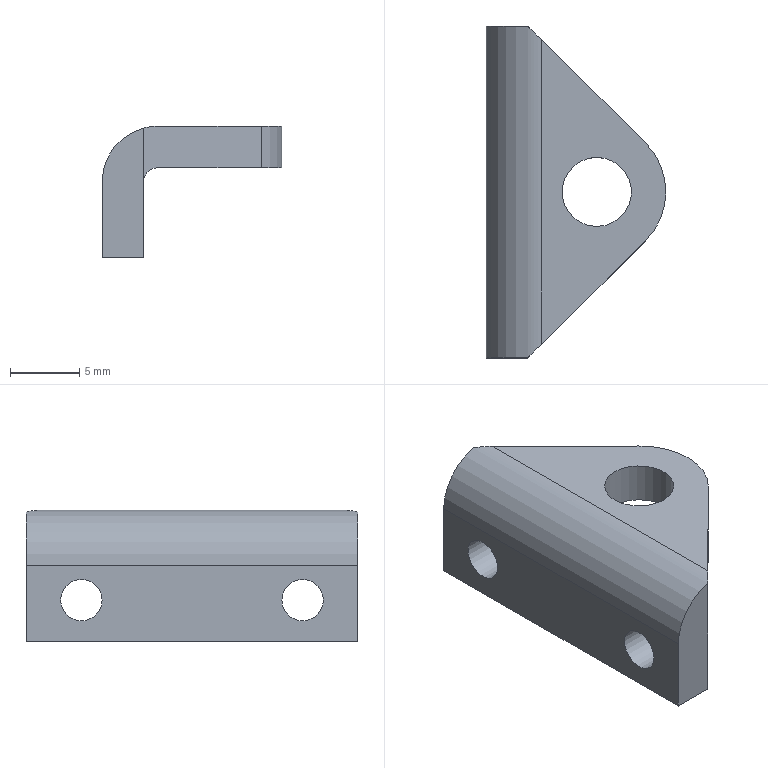Part | STEP file | 1-40.8 | 1 solid | 15 faces | box 13 x 24 x 9.5 mm | volume 924.566 mm3 | plane 9 | cylinder 6 | commonest cylinder face diameters 3 x2 2 x1 5 x1 8 x1 10 x1
STEP:
#1=CARTESIAN_POINT('',(0.,0.,0.));
#2=DIRECTION('',(0.,0.,1.));
#3=DIRECTION('',(1.,0.,0.));
#4=AXIS2_PLACEMENT_3D('',#1,#2,#3);
#5=CARTESIAN_POINT('',(0.,-12.,-4.75));
#6=VERTEX_POINT('',#5);
#7=CARTESIAN_POINT('',(0.,12.,-4.75));
#8=VERTEX_POINT('',#7);
#9=CARTESIAN_POINT('',(0.,-12.,-4.75));
#10=DIRECTION('',(0.,1.,0.));
#11=VECTOR('',#10,1.);
#12=LINE('',#9,#11);
#13=CARTESIAN_POINT('',(1.5,0.,-4.75));
#14=DIRECTION('',(0.,0.,-1.));
#15=DIRECTION('',(0.,1.,0.));
#16=AXIS2_PLACEMENT_3D('',#13,#14,#15);
#17=PLANE('',#16);
#18=CARTESIAN_POINT('',(-12.,-1.5));
#19=DIRECTION('',(1.,0.));
#20=VECTOR('',#19,1.);
#21=LINE('',#18,#20);
#22=(GEOMETRIC_REPRESENTATION_CONTEXT(2)PARAMETRIC_REPRESENTATION_CONTEXT()REPRESENTATION_CONTEXT('',''));
#23=DEFINITIONAL_REPRESENTATION('',(#21),#22);
#24=PCURVE('',#17,#23);
#25=CARTESIAN_POINT('',(0.,0.,7.25));
#26=DIRECTION('',(1.,0.,0.));
#27=DIRECTION('',(0.,1.,0.));
#28=AXIS2_PLACEMENT_3D('',#25,#26,#27);
#29=PLANE('',#28);
#30=CARTESIAN_POINT('',(-12.,-12.));
#31=DIRECTION('',(1.,0.));
#32=VECTOR('',#31,1.);
#33=LINE('',#30,#32);
#34=(GEOMETRIC_REPRESENTATION_CONTEXT(2)PARAMETRIC_REPRESENTATION_CONTEXT()REPRESENTATION_CONTEXT('',''));
#35=DEFINITIONAL_REPRESENTATION('',(#33),#34);
#36=PCURVE('',#29,#35);
#37=SURFACE_CURVE('',#12,(#24,#36),.PCURVE_S1.);
#38=EDGE_CURVE('',#6,#8,#37,.T.);
#39=ORIENTED_EDGE('',*,*,#38,.T.);
#40=CARTESIAN_POINT('',(3.,12.,-4.75));
#41=VERTEX_POINT('',#40);
#42=CARTESIAN_POINT('',(0.,12.,-4.75));
#43=DIRECTION('',(1.,0.,0.));
#44=VECTOR('',#43,1.);
#45=LINE('',#42,#44);
#46=CARTESIAN_POINT('',(12.,-1.5));
#47=DIRECTION('',(0.,1.));
#48=VECTOR('',#47,1.);
#49=LINE('',#46,#48);
#50=(GEOMETRIC_REPRESENTATION_CONTEXT(2)PARAMETRIC_REPRESENTATION_CONTEXT()REPRESENTATION_CONTEXT('',''));
#51=DEFINITIONAL_REPRESENTATION('',(#49),#50);
#52=PCURVE('',#17,#51);
#53=CARTESIAN_POINT('',(-0.375,12.,2.75));
#54=DIRECTION('',(0.,1.,0.));
#55=DIRECTION('',(0.,0.,1.));
#56=AXIS2_PLACEMENT_3D('',#53,#54,#55);
#57=PLANE('',#56);
#58=CARTESIAN_POINT('',(-7.5,0.375));
#59=DIRECTION('',(0.,1.));
#60=VECTOR('',#59,1.);
#61=LINE('',#58,#60);
#62=(GEOMETRIC_REPRESENTATION_CONTEXT(2)PARAMETRIC_REPRESENTATION_CONTEXT()REPRESENTATION_CONTEXT('',''));
#63=DEFINITIONAL_REPRESENTATION('',(#61),#62);
#64=PCURVE('',#57,#63);
#65=SURFACE_CURVE('',#45,(#52,#64),.PCURVE_S1.);
#66=EDGE_CURVE('',#8,#41,#65,.T.);
#67=ORIENTED_EDGE('',*,*,#66,.T.);
#68=CARTESIAN_POINT('',(3.,-12.,-4.75));
#69=VERTEX_POINT('',#68);
#70=CARTESIAN_POINT('',(3.,-12.,-4.75));
#71=DIRECTION('',(0.,1.,0.));
#72=VECTOR('',#71,1.);
#73=LINE('',#70,#72);
#74=CARTESIAN_POINT('',(-12.,1.5));
#75=DIRECTION('',(1.,0.));
#76=VECTOR('',#75,1.);
#77=LINE('',#74,#76);
#78=(GEOMETRIC_REPRESENTATION_CONTEXT(2)PARAMETRIC_REPRESENTATION_CONTEXT()REPRESENTATION_CONTEXT('',''));
#79=DEFINITIONAL_REPRESENTATION('',(#77),#78);
#80=PCURVE('',#17,#79);
#81=CARTESIAN_POINT('',(3.,0.,7.25));
#82=DIRECTION('',(1.,0.,0.));
#83=DIRECTION('',(0.,1.,0.));
#84=AXIS2_PLACEMENT_3D('',#81,#82,#83);
#85=PLANE('',#84);
#86=CARTESIAN_POINT('',(-12.,-12.));
#87=DIRECTION('',(1.,0.));
#88=VECTOR('',#87,1.);
#89=LINE('',#86,#88);
#90=(GEOMETRIC_REPRESENTATION_CONTEXT(2)PARAMETRIC_REPRESENTATION_CONTEXT()REPRESENTATION_CONTEXT('',''));
#91=DEFINITIONAL_REPRESENTATION('',(#89),#90);
#92=PCURVE('',#85,#91);
#93=SURFACE_CURVE('',#73,(#80,#92),.PCURVE_S1.);
#94=EDGE_CURVE('',#69,#41,#93,.T.);
#95=ORIENTED_EDGE('',*,*,#94,.F.);
#96=CARTESIAN_POINT('',(0.,-12.,-4.75));
#97=DIRECTION('',(1.,0.,0.));
#98=VECTOR('',#97,1.);
#99=LINE('',#96,#98);
#100=CARTESIAN_POINT('',(-12.,-1.5));
#101=DIRECTION('',(0.,1.));
#102=VECTOR('',#101,1.);
#103=LINE('',#100,#102);
#104=(GEOMETRIC_REPRESENTATION_CONTEXT(2)PARAMETRIC_REPRESENTATION_CONTEXT()REPRESENTATION_CONTEXT('',''));
#105=DEFINITIONAL_REPRESENTATION('',(#103),#104);
#106=PCURVE('',#17,#105);
#107=CARTESIAN_POINT('',(-0.375,-12.,2.75));
#108=DIRECTION('',(0.,-1.,0.));
#109=DIRECTION('',(0.,0.,-1.));
#110=AXIS2_PLACEMENT_3D('',#107,#108,#109);
#111=PLANE('',#110);
#112=CARTESIAN_POINT('',(7.5,0.375));
#113=DIRECTION('',(0.,1.));
#114=VECTOR('',#113,1.);
#115=LINE('',#112,#114);
#116=(GEOMETRIC_REPRESENTATION_CONTEXT(2)PARAMETRIC_REPRESENTATION_CONTEXT()REPRESENTATION_CONTEXT('',''));
#117=DEFINITIONAL_REPRESENTATION('',(#115),#116);
#118=PCURVE('',#111,#117);
#119=SURFACE_CURVE('',#99,(#106,#118),.PCURVE_S1.);
#120=EDGE_CURVE('',#6,#69,#119,.T.);
#121=ORIENTED_EDGE('',*,*,#120,.F.);
#122=EDGE_LOOP('',(#39,#67,#95,#121));
#123=FACE_BOUND('',#122,.T.);
#124=ADVANCED_FACE('',(#123),#17,.T.);
#125=CARTESIAN_POINT('',(0.,-6.5,-1.75));
#126=VERTEX_POINT('',#125);
#127=CARTESIAN_POINT('',(3.,-6.5,-1.75));
#128=VERTEX_POINT('',#127);
#129=CARTESIAN_POINT('',(0.,-6.5,-1.75));
#130=DIRECTION('',(1.,0.,0.));
#131=VECTOR('',#130,1.);
#132=LINE('',#129,#131);
#133=CARTESIAN_POINT('',(0.,-8.,-1.75));
#134=DIRECTION('',(1.,0.,0.));
#135=DIRECTION('',(0.,1.,0.));
#136=AXIS2_PLACEMENT_3D('',#133,#134,#135);
#137=CYLINDRICAL_SURFACE('',#136,1.5);
#138=CARTESIAN_POINT('',(6.283,0.));
#139=DIRECTION('',(0.,1.));
#140=VECTOR('',#139,1.);
#141=LINE('',#138,#140);
#142=(GEOMETRIC_REPRESENTATION_CONTEXT(2)PARAMETRIC_REPRESENTATION_CONTEXT()REPRESENTATION_CONTEXT('',''));
#143=DEFINITIONAL_REPRESENTATION('',(#141),#142);
#144=PCURVE('',#137,#143);
#145=CARTESIAN_POINT('',(0.,0.));
#146=DIRECTION('',(0.,1.));
#147=VECTOR('',#146,1.);
#148=LINE('',#145,#147);
#149=(GEOMETRIC_REPRESENTATION_CONTEXT(2)PARAMETRIC_REPRESENTATION_CONTEXT()REPRESENTATION_CONTEXT('',''));
#150=DEFINITIONAL_REPRESENTATION('',(#148),#149);
#151=PCURVE('',#137,#150);
#152=SEAM_CURVE('',#132,(#144,#151),.PCURVE_S1.);
#153=EDGE_CURVE('',#126,#128,#152,.T.);
#154=ORIENTED_EDGE('',*,*,#153,.T.);
#155=CARTESIAN_POINT('',(3.,-8.,-1.75));
#156=DIRECTION('',(-1.,0.,0.));
#157=DIRECTION('',(0.,1.,0.));
#158=AXIS2_PLACEMENT_3D('',#155,#156,#157);
#159=CIRCLE('',#158,1.5);
#160=CARTESIAN_POINT('',(6.283,3.));
#161=DIRECTION('',(-1.,0.));
#162=VECTOR('',#161,1.);
#163=LINE('',#160,#162);
#164=(GEOMETRIC_REPRESENTATION_CONTEXT(2)PARAMETRIC_REPRESENTATION_CONTEXT()REPRESENTATION_CONTEXT('',''));
#165=DEFINITIONAL_REPRESENTATION('',(#163),#164);
#166=PCURVE('',#137,#165);
#167=CARTESIAN_POINT('',(-6.5,-9.));
#168=CARTESIAN_POINT('',(-6.5,-11.598));
#169=CARTESIAN_POINT('',(-8.75,-10.299));
#170=CARTESIAN_POINT('',(-11.,-9.));
#171=CARTESIAN_POINT('',(-8.75,-7.701));
#172=CARTESIAN_POINT('',(-6.5,-6.402));
#173=CARTESIAN_POINT('',(-6.5,-9.));
#174=(BOUNDED_CURVE()B_SPLINE_CURVE(2,(#167,#168,#169,#170,#171,#172,#173),.UNSPECIFIED.,.T.,.F.)B_SPLINE_CURVE_WITH_KNOTS((1,2,2,2,2,1),(-2.094,0.,2.094,4.189,6.283,8.378),.UNSPECIFIED.)CURVE()GEOMETRIC_REPRESENTATION_ITEM()RATIONAL_B_SPLINE_CURVE((1.,0.5,1.,0.5,1.,0.5,1.))REPRESENTATION_ITEM(''));
#175=(GEOMETRIC_REPRESENTATION_CONTEXT(2)PARAMETRIC_REPRESENTATION_CONTEXT()REPRESENTATION_CONTEXT('',''));
#176=DEFINITIONAL_REPRESENTATION('',(#174),#175);
#177=PCURVE('',#85,#176);
#178=SURFACE_CURVE('',#159,(#166,#177),.PCURVE_S1.);
#179=EDGE_CURVE('',#128,#128,#178,.T.);
#180=ORIENTED_EDGE('',*,*,#179,.T.);
#181=ORIENTED_EDGE('',*,*,#153,.F.);
#182=CARTESIAN_POINT('',(0.,-8.,-1.75));
#183=DIRECTION('',(-1.,0.,0.));
#184=DIRECTION('',(0.,1.,0.));
#185=AXIS2_PLACEMENT_3D('',#182,#183,#184);
#186=CIRCLE('',#185,1.5);
#187=CARTESIAN_POINT('',(6.283,0.));
#188=DIRECTION('',(-1.,0.));
#189=VECTOR('',#188,1.);
#190=LINE('',#187,#189);
#191=(GEOMETRIC_REPRESENTATION_CONTEXT(2)PARAMETRIC_REPRESENTATION_CONTEXT()REPRESENTATION_CONTEXT('',''));
#192=DEFINITIONAL_REPRESENTATION('',(#190),#191);
#193=PCURVE('',#137,#192);
#194=CARTESIAN_POINT('',(-6.5,-9.));
#195=CARTESIAN_POINT('',(-6.5,-11.598));
#196=CARTESIAN_POINT('',(-8.75,-10.299));
#197=CARTESIAN_POINT('',(-11.,-9.));
#198=CARTESIAN_POINT('',(-8.75,-7.701));
#199=CARTESIAN_POINT('',(-6.5,-6.402));
#200=CARTESIAN_POINT('',(-6.5,-9.));
#201=(BOUNDED_CURVE()B_SPLINE_CURVE(2,(#194,#195,#196,#197,#198,#199,#200),.UNSPECIFIED.,.T.,.F.)B_SPLINE_CURVE_WITH_KNOTS((1,2,2,2,2,1),(-2.094,0.,2.094,4.189,6.283,8.378),.UNSPECIFIED.)CURVE()GEOMETRIC_REPRESENTATION_ITEM()RATIONAL_B_SPLINE_CURVE((1.,0.5,1.,0.5,1.,0.5,1.))REPRESENTATION_ITEM(''));
#202=(GEOMETRIC_REPRESENTATION_CONTEXT(2)PARAMETRIC_REPRESENTATION_CONTEXT()REPRESENTATION_CONTEXT('',''));
#203=DEFINITIONAL_REPRESENTATION('',(#201),#202);
#204=PCURVE('',#29,#203);
#205=SURFACE_CURVE('',#186,(#193,#204),.PCURVE_S1.);
#206=EDGE_CURVE('',#126,#126,#205,.T.);
#207=ORIENTED_EDGE('',*,*,#206,.F.);
#208=EDGE_LOOP('',(#154,#180,#181,#207));
#209=FACE_BOUND('',#208,.F.);
#210=ADVANCED_FACE('',(#209),#137,.F.);
#211=CARTESIAN_POINT('',(0.,9.5,-1.75));
#212=VERTEX_POINT('',#211);
#213=CARTESIAN_POINT('',(3.,9.5,-1.75));
#214=VERTEX_POINT('',#213);
#215=CARTESIAN_POINT('',(0.,9.5,-1.75));
#216=DIRECTION('',(1.,0.,0.));
#217=VECTOR('',#216,1.);
#218=LINE('',#215,#217);
#219=CARTESIAN_POINT('',(0.,8.,-1.75));
#220=DIRECTION('',(1.,0.,0.));
#221=DIRECTION('',(0.,1.,0.));
#222=AXIS2_PLACEMENT_3D('',#219,#220,#221);
#223=CYLINDRICAL_SURFACE('',#222,1.5);
#224=CARTESIAN_POINT('',(6.283,0.));
#225=DIRECTION('',(0.,1.));
#226=VECTOR('',#225,1.);
#227=LINE('',#224,#226);
#228=(GEOMETRIC_REPRESENTATION_CONTEXT(2)PARAMETRIC_REPRESENTATION_CONTEXT()REPRESENTATION_CONTEXT('',''));
#229=DEFINITIONAL_REPRESENTATION('',(#227),#228);
#230=PCURVE('',#223,#229);
#231=CARTESIAN_POINT('',(0.,0.));
#232=DIRECTION('',(0.,1.));
#233=VECTOR('',#232,1.);
#234=LINE('',#231,#233);
#235=(GEOMETRIC_REPRESENTATION_CONTEXT(2)PARAMETRIC_REPRESENTATION_CONTEXT()REPRESENTATION_CONTEXT('',''));
#236=DEFINITIONAL_REPRESENTATION('',(#234),#235);
#237=PCURVE('',#223,#236);
#238=SEAM_CURVE('',#218,(#230,#237),.PCURVE_S1.);
#239=EDGE_CURVE('',#212,#214,#238,.T.);
#240=ORIENTED_EDGE('',*,*,#239,.T.);
#241=CARTESIAN_POINT('',(3.,8.,-1.75));
#242=DIRECTION('',(-1.,0.,0.));
#243=DIRECTION('',(0.,1.,0.));
#244=AXIS2_PLACEMENT_3D('',#241,#242,#243);
#245=CIRCLE('',#244,1.5);
#246=CARTESIAN_POINT('',(6.283,3.));
#247=DIRECTION('',(-1.,0.));
#248=VECTOR('',#247,1.);
#249=LINE('',#246,#248);
#250=(GEOMETRIC_REPRESENTATION_CONTEXT(2)PARAMETRIC_REPRESENTATION_CONTEXT()REPRESENTATION_CONTEXT('',''));
#251=DEFINITIONAL_REPRESENTATION('',(#249),#250);
#252=PCURVE('',#223,#251);
#253=CARTESIAN_POINT('',(9.5,-9.));
#254=CARTESIAN_POINT('',(9.5,-11.598));
#255=CARTESIAN_POINT('',(7.25,-10.299));
#256=CARTESIAN_POINT('',(5.,-9.));
#257=CARTESIAN_POINT('',(7.25,-7.701));
#258=CARTESIAN_POINT('',(9.5,-6.402));
#259=CARTESIAN_POINT('',(9.5,-9.));
#260=(BOUNDED_CURVE()B_SPLINE_CURVE(2,(#253,#254,#255,#256,#257,#258,#259),.UNSPECIFIED.,.T.,.F.)B_SPLINE_CURVE_WITH_KNOTS((1,2,2,2,2,1),(-2.094,0.,2.094,4.189,6.283,8.378),.UNSPECIFIED.)CURVE()GEOMETRIC_REPRESENTATION_ITEM()RATIONAL_B_SPLINE_CURVE((1.,0.5,1.,0.5,1.,0.5,1.))REPRESENTATION_ITEM(''));
#261=(GEOMETRIC_REPRESENTATION_CONTEXT(2)PARAMETRIC_REPRESENTATION_CONTEXT()REPRESENTATION_CONTEXT('',''));
#262=DEFINITIONAL_REPRESENTATION('',(#260),#261);
#263=PCURVE('',#85,#262);
#264=SURFACE_CURVE('',#245,(#252,#263),.PCURVE_S1.);
#265=EDGE_CURVE('',#214,#214,#264,.T.);
#266=ORIENTED_EDGE('',*,*,#265,.T.);
#267=ORIENTED_EDGE('',*,*,#239,.F.);
#268=CARTESIAN_POINT('',(0.,8.,-1.75));
#269=DIRECTION('',(-1.,0.,0.));
#270=DIRECTION('',(0.,1.,0.));
#271=AXIS2_PLACEMENT_3D('',#268,#269,#270);
#272=CIRCLE('',#271,1.5);
#273=CARTESIAN_POINT('',(6.283,0.));
#274=DIRECTION('',(-1.,0.));
#275=VECTOR('',#274,1.);
#276=LINE('',#273,#275);
#277=(GEOMETRIC_REPRESENTATION_CONTEXT(2)PARAMETRIC_REPRESENTATION_CONTEXT()REPRESENTATION_CONTEXT('',''));
#278=DEFINITIONAL_REPRESENTATION('',(#276),#277);
#279=PCURVE('',#223,#278);
#280=CARTESIAN_POINT('',(9.5,-9.));
#281=CARTESIAN_POINT('',(9.5,-11.598));
#282=CARTESIAN_POINT('',(7.25,-10.299));
#283=CARTESIAN_POINT('',(5.,-9.));
#284=CARTESIAN_POINT('',(7.25,-7.701));
#285=CARTESIAN_POINT('',(9.5,-6.402));
#286=CARTESIAN_POINT('',(9.5,-9.));
#287=(BOUNDED_CURVE()B_SPLINE_CURVE(2,(#280,#281,#282,#283,#284,#285,#286),.UNSPECIFIED.,.T.,.F.)B_SPLINE_CURVE_WITH_KNOTS((1,2,2,2,2,1),(-2.094,0.,2.094,4.189,6.283,8.378),.UNSPECIFIED.)CURVE()GEOMETRIC_REPRESENTATION_ITEM()RATIONAL_B_SPLINE_CURVE((1.,0.5,1.,0.5,1.,0.5,1.))REPRESENTATION_ITEM(''));
#288=(GEOMETRIC_REPRESENTATION_CONTEXT(2)PARAMETRIC_REPRESENTATION_CONTEXT()REPRESENTATION_CONTEXT('',''));
#289=DEFINITIONAL_REPRESENTATION('',(#287),#288);
#290=PCURVE('',#29,#289);
#291=SURFACE_CURVE('',#272,(#279,#290),.PCURVE_S1.);
#292=EDGE_CURVE('',#212,#212,#291,.T.);
#293=ORIENTED_EDGE('',*,*,#292,.F.);
#294=EDGE_LOOP('',(#240,#266,#267,#293));
#295=FACE_BOUND('',#294,.F.);
#296=ADVANCED_FACE('',(#295),#223,.F.);
#297=CARTESIAN_POINT('',(11.521,-3.55,4.75));
#298=VERTEX_POINT('',#297);
#299=CARTESIAN_POINT('',(11.521,-3.55,1.75));
#300=VERTEX_POINT('',#299);
#301=CARTESIAN_POINT('',(11.521,-3.55,4.75));
#302=DIRECTION('',(0.,0.,-1.));
#303=VECTOR('',#302,1.);
#304=LINE('',#301,#303);
#305=CARTESIAN_POINT('',(8.,0.,4.75));
#306=DIRECTION('',(0.,0.,-1.));
#307=DIRECTION('',(0.7041,-0.7101,0.));
#308=AXIS2_PLACEMENT_3D('',#305,#306,#307);
#309=CYLINDRICAL_SURFACE('',#308,5.);
#310=CARTESIAN_POINT('',(6.283,0.));
#311=DIRECTION('',(0.,1.));
#312=VECTOR('',#311,1.);
#313=LINE('',#310,#312);
#314=(GEOMETRIC_REPRESENTATION_CONTEXT(2)PARAMETRIC_REPRESENTATION_CONTEXT()REPRESENTATION_CONTEXT('',''));
#315=DEFINITIONAL_REPRESENTATION('',(#313),#314);
#316=PCURVE('',#309,#315);
#317=CARTESIAN_POINT('',(6.195,-8.831,4.996));
#318=DIRECTION('',(-0.7041,0.7101,0.));
#319=DIRECTION('',(0.7101,0.7041,0.));
#320=AXIS2_PLACEMENT_3D('',#317,#318,#319);
#321=PLANE('',#320);
#322=CARTESIAN_POINT('',(7.5,0.2463));
#323=DIRECTION('',(0.,1.));
#324=VECTOR('',#323,1.);
#325=LINE('',#322,#324);
#326=(GEOMETRIC_REPRESENTATION_CONTEXT(2)PARAMETRIC_REPRESENTATION_CONTEXT()REPRESENTATION_CONTEXT('',''));
#327=DEFINITIONAL_REPRESENTATION('',(#325),#326);
#328=PCURVE('',#321,#327);
#329=SURFACE_CURVE('',#304,(#316,#328),.PCURVE_S1.);
#330=EDGE_CURVE('',#298,#300,#329,.T.);
#331=ORIENTED_EDGE('',*,*,#330,.T.);
#332=CARTESIAN_POINT('',(11.521,3.55,1.75));
#333=VERTEX_POINT('',#332);
#334=CARTESIAN_POINT('',(8.,0.,1.75));
#335=DIRECTION('',(0.,0.,1.));
#336=DIRECTION('',(0.7041,-0.7101,0.));
#337=AXIS2_PLACEMENT_3D('',#334,#335,#336);
#338=CIRCLE('',#337,5.);
#339=CARTESIAN_POINT('',(6.283,3.));
#340=DIRECTION('',(-1.,0.));
#341=VECTOR('',#340,1.);
#342=LINE('',#339,#341);
#343=(GEOMETRIC_REPRESENTATION_CONTEXT(2)PARAMETRIC_REPRESENTATION_CONTEXT()REPRESENTATION_CONTEXT('',''));
#344=DEFINITIONAL_REPRESENTATION('',(#342),#343);
#345=PCURVE('',#309,#344);
#346=CARTESIAN_POINT('',(3.101,0.,1.75));
#347=DIRECTION('',(0.,0.,1.));
#348=DIRECTION('',(0.,1.,0.));
#349=AXIS2_PLACEMENT_3D('',#346,#347,#348);
#350=PLANE('',#349);
#351=CARTESIAN_POINT('',(0.,-4.899));
#352=DIRECTION('',(-0.7101,-0.7041));
#353=AXIS2_PLACEMENT_2D('',#351,#352);
#354=CIRCLE('',#353,5.);
#355=(GEOMETRIC_REPRESENTATION_CONTEXT(2)PARAMETRIC_REPRESENTATION_CONTEXT()REPRESENTATION_CONTEXT('',''));
#356=DEFINITIONAL_REPRESENTATION('',(#354),#355);
#357=PCURVE('',#350,#356);
#358=SURFACE_CURVE('',#338,(#345,#357),.PCURVE_S1.);
#359=EDGE_CURVE('',#300,#333,#358,.T.);
#360=ORIENTED_EDGE('',*,*,#359,.T.);
#361=CARTESIAN_POINT('',(11.521,3.55,4.75));
#362=VERTEX_POINT('',#361);
#363=CARTESIAN_POINT('',(11.521,3.55,4.75));
#364=DIRECTION('',(0.,0.,-1.));
#365=VECTOR('',#364,1.);
#366=LINE('',#363,#365);
#367=CARTESIAN_POINT('',(4.704,0.));
#368=DIRECTION('',(0.,1.));
#369=VECTOR('',#368,1.);
#370=LINE('',#367,#369);
#371=(GEOMETRIC_REPRESENTATION_CONTEXT(2)PARAMETRIC_REPRESENTATION_CONTEXT()REPRESENTATION_CONTEXT('',''));
#372=DEFINITIONAL_REPRESENTATION('',(#370),#371);
#373=PCURVE('',#309,#372);
#374=CARTESIAN_POINT('',(6.195,8.831,4.996));
#375=DIRECTION('',(-0.7041,-0.7101,0.));
#376=DIRECTION('',(-0.7101,0.7041,0.));
#377=AXIS2_PLACEMENT_3D('',#374,#375,#376);
#378=PLANE('',#377);
#379=CARTESIAN_POINT('',(-7.5,0.2463));
#380=DIRECTION('',(0.,1.));
#381=VECTOR('',#380,1.);
#382=LINE('',#379,#381);
#383=(GEOMETRIC_REPRESENTATION_CONTEXT(2)PARAMETRIC_REPRESENTATION_CONTEXT()REPRESENTATION_CONTEXT('',''));
#384=DEFINITIONAL_REPRESENTATION('',(#382),#383);
#385=PCURVE('',#378,#384);
#386=SURFACE_CURVE('',#366,(#373,#385),.PCURVE_S1.);
#387=EDGE_CURVE('',#362,#333,#386,.T.);
#388=ORIENTED_EDGE('',*,*,#387,.F.);
#389=CARTESIAN_POINT('',(8.,0.,4.75));
#390=DIRECTION('',(0.,0.,1.));
#391=DIRECTION('',(0.7041,-0.7101,0.));
#392=AXIS2_PLACEMENT_3D('',#389,#390,#391);
#393=CIRCLE('',#392,5.);
#394=CARTESIAN_POINT('',(6.283,0.));
#395=DIRECTION('',(-1.,0.));
#396=VECTOR('',#395,1.);
#397=LINE('',#394,#396);
#398=(GEOMETRIC_REPRESENTATION_CONTEXT(2)PARAMETRIC_REPRESENTATION_CONTEXT()REPRESENTATION_CONTEXT('',''));
#399=DEFINITIONAL_REPRESENTATION('',(#397),#398);
#400=PCURVE('',#309,#399);
#401=CARTESIAN_POINT('',(3.101,0.,4.75));
#402=DIRECTION('',(0.,0.,1.));
#403=DIRECTION('',(0.,-1.,0.));
#404=AXIS2_PLACEMENT_3D('',#401,#402,#403);
#405=PLANE('',#404);
#406=CARTESIAN_POINT('',(0.,4.899));
#407=DIRECTION('',(0.7101,0.7041));
#408=AXIS2_PLACEMENT_2D('',#406,#407);
#409=CIRCLE('',#408,5.);
#410=(GEOMETRIC_REPRESENTATION_CONTEXT(2)PARAMETRIC_REPRESENTATION_CONTEXT()REPRESENTATION_CONTEXT('',''));
#411=DEFINITIONAL_REPRESENTATION('',(#409),#410);
#412=PCURVE('',#405,#411);
#413=SURFACE_CURVE('',#393,(#400,#412),.PCURVE_S1.);
#414=EDGE_CURVE('',#298,#362,#413,.T.);
#415=ORIENTED_EDGE('',*,*,#414,.F.);
#416=EDGE_LOOP('',(#331,#360,#388,#415));
#417=FACE_BOUND('',#416,.T.);
#418=ADVANCED_FACE('',(#417),#309,.T.);
#419=CARTESIAN_POINT('',(8.,2.5,4.75));
#420=VERTEX_POINT('',#419);
#421=CARTESIAN_POINT('',(8.,0.,4.75));
#422=DIRECTION('',(0.,0.,-1.));
#423=DIRECTION('',(0.,1.,0.));
#424=AXIS2_PLACEMENT_3D('',#421,#422,#423);
#425=CIRCLE('',#424,2.5);
#426=CARTESIAN_POINT('',(8.,0.,4.75));
#427=DIRECTION('',(0.,0.,-1.));
#428=DIRECTION('',(0.,1.,0.));
#429=AXIS2_PLACEMENT_3D('',#426,#427,#428);
#430=CYLINDRICAL_SURFACE('',#429,2.5);
#431=CARTESIAN_POINT('',(0.,0.));
#432=DIRECTION('',(1.,0.));
#433=VECTOR('',#432,1.);
#434=LINE('',#431,#433);
#435=(GEOMETRIC_REPRESENTATION_CONTEXT(2)PARAMETRIC_REPRESENTATION_CONTEXT()REPRESENTATION_CONTEXT('',''));
#436=DEFINITIONAL_REPRESENTATION('',(#434),#435);
#437=PCURVE('',#430,#436);
#438=CARTESIAN_POINT('',(-2.5,4.899));
#439=CARTESIAN_POINT('',(-2.5,9.229));
#440=CARTESIAN_POINT('',(1.25,7.064));
#441=CARTESIAN_POINT('',(5.,4.899));
#442=CARTESIAN_POINT('',(1.25,2.734));
#443=CARTESIAN_POINT('',(-2.5,0.569));
#444=CARTESIAN_POINT('',(-2.5,4.899));
#445=(BOUNDED_CURVE()B_SPLINE_CURVE(2,(#438,#439,#440,#441,#442,#443,#444),.UNSPECIFIED.,.T.,.F.)B_SPLINE_CURVE_WITH_KNOTS((1,2,2,2,2,1),(-2.094,0.,2.094,4.189,6.283,8.378),.UNSPECIFIED.)CURVE()GEOMETRIC_REPRESENTATION_ITEM()RATIONAL_B_SPLINE_CURVE((1.,0.5,1.,0.5,1.,0.5,1.))REPRESENTATION_ITEM(''));
#446=(GEOMETRIC_REPRESENTATION_CONTEXT(2)PARAMETRIC_REPRESENTATION_CONTEXT()REPRESENTATION_CONTEXT('',''));
#447=DEFINITIONAL_REPRESENTATION('',(#445),#446);
#448=PCURVE('',#405,#447);
#449=SURFACE_CURVE('',#425,(#437,#448),.PCURVE_S1.);
#450=EDGE_CURVE('',#420,#420,#449,.T.);
#451=ORIENTED_EDGE('',*,*,#450,.T.);
#452=CARTESIAN_POINT('',(8.,2.5,1.75));
#453=VERTEX_POINT('',#452);
#454=CARTESIAN_POINT('',(8.,2.5,4.75));
#455=DIRECTION('',(0.,0.,-1.));
#456=VECTOR('',#455,1.);
#457=LINE('',#454,#456);
#458=CARTESIAN_POINT('',(6.283,0.));
#459=DIRECTION('',(0.,1.));
#460=VECTOR('',#459,1.);
#461=LINE('',#458,#460);
#462=(GEOMETRIC_REPRESENTATION_CONTEXT(2)PARAMETRIC_REPRESENTATION_CONTEXT()REPRESENTATION_CONTEXT('',''));
#463=DEFINITIONAL_REPRESENTATION('',(#461),#462);
#464=PCURVE('',#430,#463);
#465=CARTESIAN_POINT('',(0.,0.));
#466=DIRECTION('',(0.,1.));
#467=VECTOR('',#466,1.);
#468=LINE('',#465,#467);
#469=(GEOMETRIC_REPRESENTATION_CONTEXT(2)PARAMETRIC_REPRESENTATION_CONTEXT()REPRESENTATION_CONTEXT('',''));
#470=DEFINITIONAL_REPRESENTATION('',(#468),#469);
#471=PCURVE('',#430,#470);
#472=SEAM_CURVE('',#457,(#464,#471),.PCURVE_S1.);
#473=EDGE_CURVE('',#420,#453,#472,.T.);
#474=ORIENTED_EDGE('',*,*,#473,.T.);
#475=CARTESIAN_POINT('',(8.,0.,1.75));
#476=DIRECTION('',(0.,0.,-1.));
#477=DIRECTION('',(0.,1.,0.));
#478=AXIS2_PLACEMENT_3D('',#475,#476,#477);
#479=CIRCLE('',#478,2.5);
#480=CARTESIAN_POINT('',(0.,3.));
#481=DIRECTION('',(1.,0.));
#482=VECTOR('',#481,1.);
#483=LINE('',#480,#482);
#484=(GEOMETRIC_REPRESENTATION_CONTEXT(2)PARAMETRIC_REPRESENTATION_CONTEXT()REPRESENTATION_CONTEXT('',''));
#485=DEFINITIONAL_REPRESENTATION('',(#483),#484);
#486=PCURVE('',#430,#485);
#487=CARTESIAN_POINT('',(2.5,-4.899));
#488=CARTESIAN_POINT('',(2.5,-9.229));
#489=CARTESIAN_POINT('',(-1.25,-7.064));
#490=CARTESIAN_POINT('',(-5.,-4.899));
#491=CARTESIAN_POINT('',(-1.25,-2.734));
#492=CARTESIAN_POINT('',(2.5,-0.569));
#493=CARTESIAN_POINT('',(2.5,-4.899));
#494=(BOUNDED_CURVE()B_SPLINE_CURVE(2,(#487,#488,#489,#490,#491,#492,#493),.UNSPECIFIED.,.T.,.F.)B_SPLINE_CURVE_WITH_KNOTS((1,2,2,2,2,1),(-2.094,0.,2.094,4.189,6.283,8.378),.UNSPECIFIED.)CURVE()GEOMETRIC_REPRESENTATION_ITEM()RATIONAL_B_SPLINE_CURVE((1.,0.5,1.,0.5,1.,0.5,1.))REPRESENTATION_ITEM(''));
#495=(GEOMETRIC_REPRESENTATION_CONTEXT(2)PARAMETRIC_REPRESENTATION_CONTEXT()REPRESENTATION_CONTEXT('',''));
#496=DEFINITIONAL_REPRESENTATION('',(#494),#495);
#497=PCURVE('',#350,#496);
#498=SURFACE_CURVE('',#479,(#486,#497),.PCURVE_S1.);
#499=EDGE_CURVE('',#453,#453,#498,.T.);
#500=ORIENTED_EDGE('',*,*,#499,.F.);
#501=ORIENTED_EDGE('',*,*,#473,.F.);
#502=EDGE_LOOP('',(#451,#474,#500,#501));
#503=FACE_BOUND('',#502,.F.);
#504=ADVANCED_FACE('',(#503),#430,.F.);
#505=ORIENTED_EDGE('',*,*,#38,.T.);
#506=CARTESIAN_POINT('',(0.,12.,0.75));
#507=VERTEX_POINT('',#506);
#508=CARTESIAN_POINT('',(0.,12.,-4.75));
#509=DIRECTION('',(0.,0.,1.));
#510=VECTOR('',#509,1.);
#511=LINE('',#508,#510);
#512=CARTESIAN_POINT('',(12.,-12.));
#513=DIRECTION('',(0.,1.));
#514=VECTOR('',#513,1.);
#515=LINE('',#512,#514);
#516=(GEOMETRIC_REPRESENTATION_CONTEXT(2)PARAMETRIC_REPRESENTATION_CONTEXT()REPRESENTATION_CONTEXT('',''));
#517=DEFINITIONAL_REPRESENTATION('',(#515),#516);
#518=PCURVE('',#29,#517);
#519=CARTESIAN_POINT('',(-7.5,0.375));
#520=DIRECTION('',(1.,0.));
#521=VECTOR('',#520,1.);
#522=LINE('',#519,#521);
#523=(GEOMETRIC_REPRESENTATION_CONTEXT(2)PARAMETRIC_REPRESENTATION_CONTEXT()REPRESENTATION_CONTEXT('',''));
#524=DEFINITIONAL_REPRESENTATION('',(#522),#523);
#525=PCURVE('',#57,#524);
#526=SURFACE_CURVE('',#511,(#518,#525),.PCURVE_S1.);
#527=EDGE_CURVE('',#8,#507,#526,.T.);
#528=ORIENTED_EDGE('',*,*,#527,.T.);
#529=CARTESIAN_POINT('',(0.,-12.,0.75));
#530=VERTEX_POINT('',#529);
#531=CARTESIAN_POINT('',(0.,12.,0.75));
#532=DIRECTION('',(0.,-1.,0.));
#533=VECTOR('',#532,1.);
#534=LINE('',#531,#533);
#535=CARTESIAN_POINT('',(12.,-6.5));
#536=DIRECTION('',(-1.,0.));
#537=VECTOR('',#536,1.);
#538=LINE('',#535,#537);
#539=(GEOMETRIC_REPRESENTATION_CONTEXT(2)PARAMETRIC_REPRESENTATION_CONTEXT()REPRESENTATION_CONTEXT('',''));
#540=DEFINITIONAL_REPRESENTATION('',(#538),#539);
#541=PCURVE('',#29,#540);
#542=CARTESIAN_POINT('',(4.,18.857,0.75));
#543=DIRECTION('',(0.,-1.,0.));
#544=DIRECTION('',(-1.,0.,0.));
#545=AXIS2_PLACEMENT_3D('',#542,#543,#544);
#546=CYLINDRICAL_SURFACE('',#545,4.);
#547=CARTESIAN_POINT('',(6.283,6.857));
#548=DIRECTION('',(0.,1.));
#549=VECTOR('',#548,1.);
#550=LINE('',#547,#549);
#551=(GEOMETRIC_REPRESENTATION_CONTEXT(2)PARAMETRIC_REPRESENTATION_CONTEXT()REPRESENTATION_CONTEXT('',''));
#552=DEFINITIONAL_REPRESENTATION('',(#550),#551);
#553=PCURVE('',#546,#552);
#554=SURFACE_CURVE('',#534,(#541,#553),.PCURVE_S1.);
#555=EDGE_CURVE('',#507,#530,#554,.T.);
#556=ORIENTED_EDGE('',*,*,#555,.T.);
#557=CARTESIAN_POINT('',(0.,-12.,0.75));
#558=DIRECTION('',(0.,0.,-1.));
#559=VECTOR('',#558,1.);
#560=LINE('',#557,#559);
#561=CARTESIAN_POINT('',(-12.,-6.5));
#562=DIRECTION('',(0.,-1.));
#563=VECTOR('',#562,1.);
#564=LINE('',#561,#563);
#565=(GEOMETRIC_REPRESENTATION_CONTEXT(2)PARAMETRIC_REPRESENTATION_CONTEXT()REPRESENTATION_CONTEXT('',''));
#566=DEFINITIONAL_REPRESENTATION('',(#564),#565);
#567=PCURVE('',#29,#566);
#568=CARTESIAN_POINT('',(2.,0.375));
#569=DIRECTION('',(1.,0.));
#570=VECTOR('',#569,1.);
#571=LINE('',#568,#570);
#572=(GEOMETRIC_REPRESENTATION_CONTEXT(2)PARAMETRIC_REPRESENTATION_CONTEXT()REPRESENTATION_CONTEXT('',''));
#573=DEFINITIONAL_REPRESENTATION('',(#571),#572);
#574=PCURVE('',#111,#573);
#575=SURFACE_CURVE('',#560,(#567,#574),.PCURVE_S1.);
#576=EDGE_CURVE('',#530,#6,#575,.T.);
#577=ORIENTED_EDGE('',*,*,#576,.T.);
#578=EDGE_LOOP('',(#505,#528,#556,#577));
#579=FACE_BOUND('',#578,.F.);
#580=ORIENTED_EDGE('',*,*,#292,.T.);
#581=EDGE_LOOP('',(#580));
#582=FACE_BOUND('',#581,.F.);
#583=ORIENTED_EDGE('',*,*,#206,.T.);
#584=EDGE_LOOP('',(#583));
#585=FACE_BOUND('',#584,.F.);
#586=ADVANCED_FACE('',(#579,#582,#585),#29,.F.);
#587=ORIENTED_EDGE('',*,*,#414,.T.);
#588=CARTESIAN_POINT('',(4.,11.008,4.75));
#589=VERTEX_POINT('',#588);
#590=CARTESIAN_POINT('',(11.521,3.55,4.75));
#591=DIRECTION('',(-0.7101,0.7041,0.));
#592=VECTOR('',#591,1.);
#593=LINE('',#590,#592);
#594=CARTESIAN_POINT('',(-3.55,8.42));
#595=DIRECTION('',(-0.7041,-0.7101));
#596=VECTOR('',#595,1.);
#597=LINE('',#594,#596);
#598=(GEOMETRIC_REPRESENTATION_CONTEXT(2)PARAMETRIC_REPRESENTATION_CONTEXT()REPRESENTATION_CONTEXT('',''));
#599=DEFINITIONAL_REPRESENTATION('',(#597),#598);
#600=PCURVE('',#405,#599);
#601=CARTESIAN_POINT('',(-7.5,0.2463));
#602=DIRECTION('',(1.,0.));
#603=VECTOR('',#602,1.);
#604=LINE('',#601,#603);
#605=(GEOMETRIC_REPRESENTATION_CONTEXT(2)PARAMETRIC_REPRESENTATION_CONTEXT()REPRESENTATION_CONTEXT('',''));
#606=DEFINITIONAL_REPRESENTATION('',(#604),#605);
#607=PCURVE('',#378,#606);
#608=SURFACE_CURVE('',#593,(#600,#607),.PCURVE_S1.);
#609=EDGE_CURVE('',#362,#589,#608,.T.);
#610=ORIENTED_EDGE('',*,*,#609,.T.);
#611=CARTESIAN_POINT('',(4.,-11.008,4.75));
#612=VERTEX_POINT('',#611);
#613=CARTESIAN_POINT('',(4.,11.008,4.75));
#614=DIRECTION('',(0.,-1.,0.));
#615=VECTOR('',#614,1.);
#616=LINE('',#613,#615);
#617=CARTESIAN_POINT('',(-11.008,0.8992));
#618=DIRECTION('',(1.,0.));
#619=VECTOR('',#618,1.);
#620=LINE('',#617,#619);
#621=(GEOMETRIC_REPRESENTATION_CONTEXT(2)PARAMETRIC_REPRESENTATION_CONTEXT()REPRESENTATION_CONTEXT('',''));
#622=DEFINITIONAL_REPRESENTATION('',(#620),#621);
#623=PCURVE('',#405,#622);
#624=CARTESIAN_POINT('',(4.712,7.849));
#625=DIRECTION('',(0.,1.));
#626=VECTOR('',#625,1.);
#627=LINE('',#624,#626);
#628=(GEOMETRIC_REPRESENTATION_CONTEXT(2)PARAMETRIC_REPRESENTATION_CONTEXT()REPRESENTATION_CONTEXT('',''));
#629=DEFINITIONAL_REPRESENTATION('',(#627),#628);
#630=PCURVE('',#546,#629);
#631=SURFACE_CURVE('',#616,(#623,#630),.PCURVE_S1.);
#632=EDGE_CURVE('',#589,#612,#631,.T.);
#633=ORIENTED_EDGE('',*,*,#632,.T.);
#634=CARTESIAN_POINT('',(4.,-11.008,4.75));
#635=DIRECTION('',(0.7101,0.7041,0.));
#636=VECTOR('',#635,1.);
#637=LINE('',#634,#636);
#638=CARTESIAN_POINT('',(11.008,0.8992));
#639=DIRECTION('',(-0.7041,0.7101));
#640=VECTOR('',#639,1.);
#641=LINE('',#638,#640);
#642=(GEOMETRIC_REPRESENTATION_CONTEXT(2)PARAMETRIC_REPRESENTATION_CONTEXT()REPRESENTATION_CONTEXT('',''));
#643=DEFINITIONAL_REPRESENTATION('',(#641),#642);
#644=PCURVE('',#405,#643);
#645=CARTESIAN_POINT('',(-3.092,0.2463));
#646=DIRECTION('',(1.,0.));
#647=VECTOR('',#646,1.);
#648=LINE('',#645,#647);
#649=(GEOMETRIC_REPRESENTATION_CONTEXT(2)PARAMETRIC_REPRESENTATION_CONTEXT()REPRESENTATION_CONTEXT('',''));
#650=DEFINITIONAL_REPRESENTATION('',(#648),#649);
#651=PCURVE('',#321,#650);
#652=SURFACE_CURVE('',#637,(#644,#651),.PCURVE_S1.);
#653=EDGE_CURVE('',#612,#298,#652,.T.);
#654=ORIENTED_EDGE('',*,*,#653,.T.);
#655=EDGE_LOOP('',(#587,#610,#633,#654));
#656=FACE_BOUND('',#655,.T.);
#657=ORIENTED_EDGE('',*,*,#450,.T.);
#658=EDGE_LOOP('',(#657));
#659=FACE_BOUND('',#658,.T.);
#660=ADVANCED_FACE('',(#656,#659),#405,.T.);
#661=ORIENTED_EDGE('',*,*,#527,.T.);
#662=CARTESIAN_POINT('',(3.,12.,4.623));
#663=VERTEX_POINT('',#662);
#664=CARTESIAN_POINT('',(4.,12.,0.75));
#665=DIRECTION('',(0.,1.,0.));
#666=DIRECTION('',(-1.,0.,0.));
#667=AXIS2_PLACEMENT_3D('',#664,#665,#666);
#668=CIRCLE('',#667,4.);
#669=CARTESIAN_POINT('',(-2.,4.375));
#670=DIRECTION('',(0.,-1.));
#671=AXIS2_PLACEMENT_2D('',#669,#670);
#672=CIRCLE('',#671,4.);
#673=(GEOMETRIC_REPRESENTATION_CONTEXT(2)PARAMETRIC_REPRESENTATION_CONTEXT()REPRESENTATION_CONTEXT('',''));
#674=DEFINITIONAL_REPRESENTATION('',(#672),#673);
#675=PCURVE('',#57,#674);
#676=CARTESIAN_POINT('',(6.283,6.857));
#677=DIRECTION('',(-1.,0.));
#678=VECTOR('',#677,1.);
#679=LINE('',#676,#678);
#680=(GEOMETRIC_REPRESENTATION_CONTEXT(2)PARAMETRIC_REPRESENTATION_CONTEXT()REPRESENTATION_CONTEXT('',''));
#681=DEFINITIONAL_REPRESENTATION('',(#679),#680);
#682=PCURVE('',#546,#681);
#683=SURFACE_CURVE('',#668,(#675,#682),.PCURVE_S1.);
#684=EDGE_CURVE('',#507,#663,#683,.T.);
#685=ORIENTED_EDGE('',*,*,#684,.T.);
#686=CARTESIAN_POINT('',(3.,12.,0.75));
#687=VERTEX_POINT('',#686);
#688=CARTESIAN_POINT('',(3.,12.,0.75));
#689=DIRECTION('',(0.,0.,1.));
#690=VECTOR('',#689,1.);
#691=LINE('',#688,#690);
#692=CARTESIAN_POINT('',(-2.,3.375));
#693=DIRECTION('',(1.,0.));
#694=VECTOR('',#693,1.);
#695=LINE('',#692,#694);
#696=(GEOMETRIC_REPRESENTATION_CONTEXT(2)PARAMETRIC_REPRESENTATION_CONTEXT()REPRESENTATION_CONTEXT('',''));
#697=DEFINITIONAL_REPRESENTATION('',(#695),#696);
#698=PCURVE('',#57,#697);
#699=CARTESIAN_POINT('',(4.5,4.246));
#700=DIRECTION('',(0.,-1.));
#701=VECTOR('',#700,1.);
#702=LINE('',#699,#701);
#703=(GEOMETRIC_REPRESENTATION_CONTEXT(2)PARAMETRIC_REPRESENTATION_CONTEXT()REPRESENTATION_CONTEXT('',''));
#704=DEFINITIONAL_REPRESENTATION('',(#702),#703);
#705=PCURVE('',#378,#704);
#706=SURFACE_CURVE('',#691,(#698,#705),.PCURVE_S1.);
#707=EDGE_CURVE('',#687,#663,#706,.T.);
#708=ORIENTED_EDGE('',*,*,#707,.F.);
#709=CARTESIAN_POINT('',(3.,12.,-4.75));
#710=DIRECTION('',(0.,0.,1.));
#711=VECTOR('',#710,1.);
#712=LINE('',#709,#711);
#713=CARTESIAN_POINT('',(-7.5,3.375));
#714=DIRECTION('',(1.,0.));
#715=VECTOR('',#714,1.);
#716=LINE('',#713,#715);
#717=(GEOMETRIC_REPRESENTATION_CONTEXT(2)PARAMETRIC_REPRESENTATION_CONTEXT()REPRESENTATION_CONTEXT('',''));
#718=DEFINITIONAL_REPRESENTATION('',(#716),#717);
#719=PCURVE('',#57,#718);
#720=CARTESIAN_POINT('',(12.,-12.));
#721=DIRECTION('',(0.,1.));
#722=VECTOR('',#721,1.);
#723=LINE('',#720,#722);
#724=(GEOMETRIC_REPRESENTATION_CONTEXT(2)PARAMETRIC_REPRESENTATION_CONTEXT()REPRESENTATION_CONTEXT('',''));
#725=DEFINITIONAL_REPRESENTATION('',(#723),#724);
#726=PCURVE('',#85,#725);
#727=SURFACE_CURVE('',#712,(#719,#726),.PCURVE_S1.);
#728=EDGE_CURVE('',#41,#687,#727,.T.);
#729=ORIENTED_EDGE('',*,*,#728,.F.);
#730=ORIENTED_EDGE('',*,*,#66,.F.);
#731=EDGE_LOOP('',(#661,#685,#708,#729,#730));
#732=FACE_BOUND('',#731,.T.);
#733=ADVANCED_FACE('',(#732),#57,.T.);
#734=CARTESIAN_POINT('',(3.,-12.,0.75));
#735=VERTEX_POINT('',#734);
#736=CARTESIAN_POINT('',(3.,-12.,0.75));
#737=DIRECTION('',(0.,0.,-1.));
#738=VECTOR('',#737,1.);
#739=LINE('',#736,#738);
#740=CARTESIAN_POINT('',(2.,3.375));
#741=DIRECTION('',(1.,0.));
#742=VECTOR('',#741,1.);
#743=LINE('',#740,#742);
#744=(GEOMETRIC_REPRESENTATION_CONTEXT(2)PARAMETRIC_REPRESENTATION_CONTEXT()REPRESENTATION_CONTEXT('',''));
#745=DEFINITIONAL_REPRESENTATION('',(#743),#744);
#746=PCURVE('',#111,#745);
#747=CARTESIAN_POINT('',(-12.,-6.5));
#748=DIRECTION('',(0.,-1.));
#749=VECTOR('',#748,1.);
#750=LINE('',#747,#749);
#751=(GEOMETRIC_REPRESENTATION_CONTEXT(2)PARAMETRIC_REPRESENTATION_CONTEXT()REPRESENTATION_CONTEXT('',''));
#752=DEFINITIONAL_REPRESENTATION('',(#750),#751);
#753=PCURVE('',#85,#752);
#754=SURFACE_CURVE('',#739,(#746,#753),.PCURVE_S1.);
#755=EDGE_CURVE('',#735,#69,#754,.T.);
#756=ORIENTED_EDGE('',*,*,#755,.F.);
#757=CARTESIAN_POINT('',(3.,-12.,4.623));
#758=VERTEX_POINT('',#757);
#759=CARTESIAN_POINT('',(3.,-12.,4.623));
#760=DIRECTION('',(0.,0.,-1.));
#761=VECTOR('',#760,1.);
#762=LINE('',#759,#761);
#763=CARTESIAN_POINT('',(-1.873,3.375));
#764=DIRECTION('',(1.,0.));
#765=VECTOR('',#764,1.);
#766=LINE('',#763,#765);
#767=(GEOMETRIC_REPRESENTATION_CONTEXT(2)PARAMETRIC_REPRESENTATION_CONTEXT()REPRESENTATION_CONTEXT('',''));
#768=DEFINITIONAL_REPRESENTATION('',(#766),#767);
#769=PCURVE('',#111,#768);
#770=CARTESIAN_POINT('',(-4.5,0.3733));
#771=DIRECTION('',(0.,1.));
#772=VECTOR('',#771,1.);
#773=LINE('',#770,#772);
#774=(GEOMETRIC_REPRESENTATION_CONTEXT(2)PARAMETRIC_REPRESENTATION_CONTEXT()REPRESENTATION_CONTEXT('',''));
#775=DEFINITIONAL_REPRESENTATION('',(#773),#774);
#776=PCURVE('',#321,#775);
#777=SURFACE_CURVE('',#762,(#769,#776),.PCURVE_S1.);
#778=EDGE_CURVE('',#758,#735,#777,.T.);
#779=ORIENTED_EDGE('',*,*,#778,.F.);
#780=CARTESIAN_POINT('',(4.,-12.,0.75));
#781=DIRECTION('',(0.,-1.,0.));
#782=DIRECTION('',(-0.25,0.,0.9682));
#783=AXIS2_PLACEMENT_3D('',#780,#781,#782);
#784=CIRCLE('',#783,4.);
#785=CARTESIAN_POINT('',(2.,4.375));
#786=DIRECTION('',(-0.9682,-0.25));
#787=AXIS2_PLACEMENT_2D('',#785,#786);
#788=CIRCLE('',#787,4.);
#789=(GEOMETRIC_REPRESENTATION_CONTEXT(2)PARAMETRIC_REPRESENTATION_CONTEXT()REPRESENTATION_CONTEXT('',''));
#790=DEFINITIONAL_REPRESENTATION('',(#788),#789);
#791=PCURVE('',#111,#790);
#792=CARTESIAN_POINT('',(4.965,30.857));
#793=DIRECTION('',(1.,0.));
#794=VECTOR('',#793,1.);
#795=LINE('',#792,#794);
#796=(GEOMETRIC_REPRESENTATION_CONTEXT(2)PARAMETRIC_REPRESENTATION_CONTEXT()REPRESENTATION_CONTEXT('',''));
#797=DEFINITIONAL_REPRESENTATION('',(#795),#796);
#798=PCURVE('',#546,#797);
#799=SURFACE_CURVE('',#784,(#791,#798),.PCURVE_S1.);
#800=EDGE_CURVE('',#758,#530,#799,.T.);
#801=ORIENTED_EDGE('',*,*,#800,.T.);
#802=ORIENTED_EDGE('',*,*,#576,.T.);
#803=ORIENTED_EDGE('',*,*,#120,.T.);
#804=EDGE_LOOP('',(#756,#779,#801,#802,#803));
#805=FACE_BOUND('',#804,.T.);
#806=ADVANCED_FACE('',(#805),#111,.T.);
#807=ORIENTED_EDGE('',*,*,#800,.F.);
#808=CARTESIAN_POINT('',(4.,-11.008,0.75));
#809=DIRECTION('',(0.7041,-0.7101,0.));
#810=DIRECTION('',(-0.7101,-0.7041,0.));
#811=AXIS2_PLACEMENT_3D('',#808,#809,#810);
#812=ELLIPSE('',#811,5.633,4.);
#813=CARTESIAN_POINT('',(4.712,29.865));
#814=CARTESIAN_POINT('',(4.965,30.857));
#815=B_SPLINE_CURVE_WITH_KNOTS('',1,(#813,#814),.UNSPECIFIED.,.F.,.F.,(2,2),(4.712,4.965),.PIECEWISE_BEZIER_KNOTS.);
#816=(GEOMETRIC_REPRESENTATION_CONTEXT(2)PARAMETRIC_REPRESENTATION_CONTEXT()REPRESENTATION_CONTEXT('',''));
#817=DEFINITIONAL_REPRESENTATION('',(#815),#816);
#818=PCURVE('',#546,#817);
#819=CARTESIAN_POINT('',(-8.725,4.246));
#820=CARTESIAN_POINT('',(-8.725,11.175));
#821=CARTESIAN_POINT('',(-0.275,7.71));
#822=CARTESIAN_POINT('',(8.175,4.246));
#823=CARTESIAN_POINT('',(-0.275,0.7822));
#824=CARTESIAN_POINT('',(-8.725,-2.682));
#825=CARTESIAN_POINT('',(-8.725,4.246));
#826=(BOUNDED_CURVE()B_SPLINE_CURVE(2,(#819,#820,#821,#822,#823,#824,#825),.UNSPECIFIED.,.T.,.F.)B_SPLINE_CURVE_WITH_KNOTS((1,2,2,2,2,1),(-2.094,0.,2.094,4.189,6.283,8.378),.UNSPECIFIED.)CURVE()GEOMETRIC_REPRESENTATION_ITEM()RATIONAL_B_SPLINE_CURVE((1.,0.5,1.,0.5,1.,0.5,1.))REPRESENTATION_ITEM(''));
#827=(GEOMETRIC_REPRESENTATION_CONTEXT(2)PARAMETRIC_REPRESENTATION_CONTEXT()REPRESENTATION_CONTEXT('',''));
#828=DEFINITIONAL_REPRESENTATION('',(#826),#827);
#829=PCURVE('',#321,#828);
#830=SURFACE_CURVE('',#812,(#818,#829),.PCURVE_S1.);
#831=EDGE_CURVE('',#612,#758,#830,.T.);
#832=ORIENTED_EDGE('',*,*,#831,.F.);
#833=ORIENTED_EDGE('',*,*,#632,.F.);
#834=CARTESIAN_POINT('',(4.,11.008,0.75));
#835=DIRECTION('',(0.7041,0.7101,0.));
#836=DIRECTION('',(-0.7101,0.7041,0.));
#837=AXIS2_PLACEMENT_3D('',#834,#835,#836);
#838=ELLIPSE('',#837,5.633,4.);
#839=CARTESIAN_POINT('',(4.965,6.857));
#840=CARTESIAN_POINT('',(4.712,7.849));
#841=B_SPLINE_CURVE_WITH_KNOTS('',1,(#839,#840),.UNSPECIFIED.,.F.,.F.,(2,2),(1.318,1.571),.PIECEWISE_BEZIER_KNOTS.);
#842=(GEOMETRIC_REPRESENTATION_CONTEXT(2)PARAMETRIC_REPRESENTATION_CONTEXT()REPRESENTATION_CONTEXT('',''));
#843=DEFINITIONAL_REPRESENTATION('',(#841),#842);
#844=PCURVE('',#546,#843);
#845=CARTESIAN_POINT('',(8.725,4.246));
#846=CARTESIAN_POINT('',(8.725,-2.682));
#847=CARTESIAN_POINT('',(0.275,0.7822));
#848=CARTESIAN_POINT('',(-8.175,4.246));
#849=CARTESIAN_POINT('',(0.275,7.71));
#850=CARTESIAN_POINT('',(8.725,11.175));
#851=CARTESIAN_POINT('',(8.725,4.246));
#852=(BOUNDED_CURVE()B_SPLINE_CURVE(2,(#845,#846,#847,#848,#849,#850,#851),.UNSPECIFIED.,.T.,.F.)B_SPLINE_CURVE_WITH_KNOTS((1,2,2,2,2,1),(-2.094,0.,2.094,4.189,6.283,8.378),.UNSPECIFIED.)CURVE()GEOMETRIC_REPRESENTATION_ITEM()RATIONAL_B_SPLINE_CURVE((1.,0.5,1.,0.5,1.,0.5,1.))REPRESENTATION_ITEM(''));
#853=(GEOMETRIC_REPRESENTATION_CONTEXT(2)PARAMETRIC_REPRESENTATION_CONTEXT()REPRESENTATION_CONTEXT('',''));
#854=DEFINITIONAL_REPRESENTATION('',(#852),#853);
#855=PCURVE('',#378,#854);
#856=SURFACE_CURVE('',#838,(#844,#855),.PCURVE_S1.);
#857=EDGE_CURVE('',#663,#589,#856,.T.);
#858=ORIENTED_EDGE('',*,*,#857,.F.);
#859=ORIENTED_EDGE('',*,*,#684,.F.);
#860=ORIENTED_EDGE('',*,*,#555,.T.);
#861=EDGE_LOOP('',(#807,#832,#833,#858,#859,#860));
#862=FACE_BOUND('',#861,.T.);
#863=ADVANCED_FACE('',(#862),#546,.T.);
#864=ORIENTED_EDGE('',*,*,#94,.T.);
#865=ORIENTED_EDGE('',*,*,#728,.T.);
#866=CARTESIAN_POINT('',(3.,12.,0.75));
#867=DIRECTION('',(0.,-1.,0.));
#868=VECTOR('',#867,1.);
#869=LINE('',#866,#868);
#870=CARTESIAN_POINT('',(12.,-6.5));
#871=DIRECTION('',(-1.,0.));
#872=VECTOR('',#871,1.);
#873=LINE('',#870,#872);
#874=(GEOMETRIC_REPRESENTATION_CONTEXT(2)PARAMETRIC_REPRESENTATION_CONTEXT()REPRESENTATION_CONTEXT('',''));
#875=DEFINITIONAL_REPRESENTATION('',(#873),#874);
#876=PCURVE('',#85,#875);
#877=CARTESIAN_POINT('',(4.,13.2,0.75));
#878=DIRECTION('',(0.,-1.,0.));
#879=DIRECTION('',(0.,0.,1.));
#880=AXIS2_PLACEMENT_3D('',#877,#878,#879);
#881=CYLINDRICAL_SURFACE('',#880,1.);
#882=CARTESIAN_POINT('',(1.571,1.2));
#883=DIRECTION('',(0.,1.));
#884=VECTOR('',#883,1.);
#885=LINE('',#882,#884);
#886=(GEOMETRIC_REPRESENTATION_CONTEXT(2)PARAMETRIC_REPRESENTATION_CONTEXT()REPRESENTATION_CONTEXT('',''));
#887=DEFINITIONAL_REPRESENTATION('',(#885),#886);
#888=PCURVE('',#881,#887);
#889=SURFACE_CURVE('',#869,(#876,#888),.PCURVE_S1.);
#890=EDGE_CURVE('',#687,#735,#889,.T.);
#891=ORIENTED_EDGE('',*,*,#890,.T.);
#892=ORIENTED_EDGE('',*,*,#755,.T.);
#893=EDGE_LOOP('',(#864,#865,#891,#892));
#894=FACE_BOUND('',#893,.T.);
#895=ORIENTED_EDGE('',*,*,#265,.T.);
#896=EDGE_LOOP('',(#895));
#897=FACE_BOUND('',#896,.T.);
#898=ORIENTED_EDGE('',*,*,#179,.T.);
#899=EDGE_LOOP('',(#898));
#900=FACE_BOUND('',#899,.T.);
#901=ADVANCED_FACE('',(#894,#897,#900),#85,.T.);
#902=ORIENTED_EDGE('',*,*,#359,.T.);
#903=CARTESIAN_POINT('',(4.,11.008,1.75));
#904=VERTEX_POINT('',#903);
#905=CARTESIAN_POINT('',(11.521,3.55,1.75));
#906=DIRECTION('',(-0.7101,0.7041,0.));
#907=VECTOR('',#906,1.);
#908=LINE('',#905,#907);
#909=CARTESIAN_POINT('',(3.55,-8.42));
#910=DIRECTION('',(0.7041,0.7101));
#911=VECTOR('',#910,1.);
#912=LINE('',#909,#911);
#913=(GEOMETRIC_REPRESENTATION_CONTEXT(2)PARAMETRIC_REPRESENTATION_CONTEXT()REPRESENTATION_CONTEXT('',''));
#914=DEFINITIONAL_REPRESENTATION('',(#912),#913);
#915=PCURVE('',#350,#914);
#916=CARTESIAN_POINT('',(-7.5,3.246));
#917=DIRECTION('',(1.,0.));
#918=VECTOR('',#917,1.);
#919=LINE('',#916,#918);
#920=(GEOMETRIC_REPRESENTATION_CONTEXT(2)PARAMETRIC_REPRESENTATION_CONTEXT()REPRESENTATION_CONTEXT('',''));
#921=DEFINITIONAL_REPRESENTATION('',(#919),#920);
#922=PCURVE('',#378,#921);
#923=SURFACE_CURVE('',#908,(#915,#922),.PCURVE_S1.);
#924=EDGE_CURVE('',#333,#904,#923,.T.);
#925=ORIENTED_EDGE('',*,*,#924,.T.);
#926=CARTESIAN_POINT('',(4.,-11.008,1.75));
#927=VERTEX_POINT('',#926);
#928=CARTESIAN_POINT('',(4.,11.008,1.75));
#929=DIRECTION('',(0.,-1.,0.));
#930=VECTOR('',#929,1.);
#931=LINE('',#928,#930);
#932=CARTESIAN_POINT('',(11.008,-0.8992));
#933=DIRECTION('',(-1.,0.));
#934=VECTOR('',#933,1.);
#935=LINE('',#932,#934);
#936=(GEOMETRIC_REPRESENTATION_CONTEXT(2)PARAMETRIC_REPRESENTATION_CONTEXT()REPRESENTATION_CONTEXT('',''));
#937=DEFINITIONAL_REPRESENTATION('',(#935),#936);
#938=PCURVE('',#350,#937);
#939=CARTESIAN_POINT('',(0.,2.192));
#940=DIRECTION('',(0.,1.));
#941=VECTOR('',#940,1.);
#942=LINE('',#939,#941);
#943=(GEOMETRIC_REPRESENTATION_CONTEXT(2)PARAMETRIC_REPRESENTATION_CONTEXT()REPRESENTATION_CONTEXT('',''));
#944=DEFINITIONAL_REPRESENTATION('',(#942),#943);
#945=PCURVE('',#881,#944);
#946=SURFACE_CURVE('',#931,(#938,#945),.PCURVE_S1.);
#947=EDGE_CURVE('',#904,#927,#946,.T.);
#948=ORIENTED_EDGE('',*,*,#947,.T.);
#949=CARTESIAN_POINT('',(4.,-11.008,1.75));
#950=DIRECTION('',(0.7101,0.7041,0.));
#951=VECTOR('',#950,1.);
#952=LINE('',#949,#951);
#953=CARTESIAN_POINT('',(-11.008,-0.8992));
#954=DIRECTION('',(0.7041,-0.7101));
#955=VECTOR('',#954,1.);
#956=LINE('',#953,#955);
#957=(GEOMETRIC_REPRESENTATION_CONTEXT(2)PARAMETRIC_REPRESENTATION_CONTEXT()REPRESENTATION_CONTEXT('',''));
#958=DEFINITIONAL_REPRESENTATION('',(#956),#957);
#959=PCURVE('',#350,#958);
#960=CARTESIAN_POINT('',(-3.092,3.246));
#961=DIRECTION('',(1.,0.));
#962=VECTOR('',#961,1.);
#963=LINE('',#960,#962);
#964=(GEOMETRIC_REPRESENTATION_CONTEXT(2)PARAMETRIC_REPRESENTATION_CONTEXT()REPRESENTATION_CONTEXT('',''));
#965=DEFINITIONAL_REPRESENTATION('',(#963),#964);
#966=PCURVE('',#321,#965);
#967=SURFACE_CURVE('',#952,(#959,#966),.PCURVE_S1.);
#968=EDGE_CURVE('',#927,#300,#967,.T.);
#969=ORIENTED_EDGE('',*,*,#968,.T.);
#970=EDGE_LOOP('',(#902,#925,#948,#969));
#971=FACE_BOUND('',#970,.F.);
#972=ORIENTED_EDGE('',*,*,#499,.T.);
#973=EDGE_LOOP('',(#972));
#974=FACE_BOUND('',#973,.F.);
#975=ADVANCED_FACE('',(#971,#974),#350,.F.);
#976=ORIENTED_EDGE('',*,*,#924,.F.);
#977=ORIENTED_EDGE('',*,*,#387,.F.);
#978=ORIENTED_EDGE('',*,*,#609,.T.);
#979=ORIENTED_EDGE('',*,*,#857,.F.);
#980=ORIENTED_EDGE('',*,*,#707,.F.);
#981=CARTESIAN_POINT('',(4.,11.008,1.75));
#982=CARTESIAN_POINT('',(3.646,11.359,1.75));
#983=CARTESIAN_POINT('',(3.213,11.789,1.547));
#984=CARTESIAN_POINT('',(3.019,11.982,0.9692));
#985=CARTESIAN_POINT('',(3.,12.,0.8616));
#986=CARTESIAN_POINT('',(3.,12.,0.75));
#987=B_SPLINE_CURVE_WITH_KNOTS('',3,(#981,#982,#983,#984,#985,#986),.UNSPECIFIED.,.F.,.F.,(4,2,4),(0.,1.,1.209),.UNSPECIFIED.);
#988=CARTESIAN_POINT('',(3.092,3.246));
#989=CARTESIAN_POINT('',(3.59,3.246));
#990=CARTESIAN_POINT('',(4.2,3.449));
#991=CARTESIAN_POINT('',(4.474,4.027));
#992=CARTESIAN_POINT('',(4.5,4.135));
#993=CARTESIAN_POINT('',(4.5,4.246));
#994=B_SPLINE_CURVE_WITH_KNOTS('',3,(#988,#989,#990,#991,#992,#993),.UNSPECIFIED.,.F.,.F.,(4,2,4),(0.,1.,1.209),.UNSPECIFIED.);
#995=(GEOMETRIC_REPRESENTATION_CONTEXT(2)PARAMETRIC_REPRESENTATION_CONTEXT()REPRESENTATION_CONTEXT('',''));
#996=DEFINITIONAL_REPRESENTATION('',(#994),#995);
#997=PCURVE('',#378,#996);
#998=CARTESIAN_POINT('',(0.,2.192));
#999=CARTESIAN_POINT('',(0.01945,2.172));
#1000=CARTESIAN_POINT('',(0.05882,2.133));
#1001=CARTESIAN_POINT('',(0.1192,2.074));
#1002=CARTESIAN_POINT('',(0.1808,2.013));
#1003=CARTESIAN_POINT('',(0.2434,1.953));
#1004=CARTESIAN_POINT('',(0.3071,1.892));
#1005=CARTESIAN_POINT('',(0.3717,1.831));
#1006=CARTESIAN_POINT('',(0.4371,1.772));
#1007=CARTESIAN_POINT('',(0.5033,1.713));
#1008=CARTESIAN_POINT('',(0.5702,1.655));
#1009=CARTESIAN_POINT('',(0.638,1.6));
#1010=CARTESIAN_POINT('',(0.7067,1.546));
#1011=CARTESIAN_POINT('',(0.7764,1.495));
#1012=CARTESIAN_POINT('',(0.8473,1.446));
#1013=CARTESIAN_POINT('',(0.9196,1.401));
#1014=CARTESIAN_POINT('',(0.9936,1.359));
#1015=CARTESIAN_POINT('',(1.07,1.32));
#1016=CARTESIAN_POINT('',(1.148,1.286));
#1017=CARTESIAN_POINT('',(1.229,1.256));
#1018=CARTESIAN_POINT('',(1.313,1.232));
#1019=CARTESIAN_POINT('',(1.397,1.214));
#1020=CARTESIAN_POINT('',(1.483,1.203));
#1021=CARTESIAN_POINT('',(1.541,1.2));
#1022=CARTESIAN_POINT('',(1.571,1.2));
#1023=B_SPLINE_CURVE_WITH_KNOTS('',3,(#998,#999,#1000,#1001,#1002,#1003,#1004,#1005,#1006,#1007,#1008,#1009,#1010,#1011,#1012,#1013,#1014,#1015,#1016,#1017,#1018,#1019,#1020,#1021,#1022),.UNSPECIFIED.,.F.,.F.,(4,1,1,1,1,1,1,1,1,1,1,1,1,1,1,1,1,1,1,1,1,1,4),(0.,0.05494,0.1099,0.1648,0.2198,0.2747,0.3296,0.3846,0.4395,0.4945,0.5494,0.6043,0.6593,0.7142,0.7692,0.8241,0.879,0.934,0.9889,1.044,1.099,1.154,1.209),.QUASI_UNIFORM_KNOTS.);
#1024=(GEOMETRIC_REPRESENTATION_CONTEXT(2)PARAMETRIC_REPRESENTATION_CONTEXT()REPRESENTATION_CONTEXT('',''));
#1025=DEFINITIONAL_REPRESENTATION('',(#1023),#1024);
#1026=PCURVE('',#881,#1025);
#1027=SURFACE_CURVE('',#987,(#997,#1026),.PCURVE_S1.);
#1028=EDGE_CURVE('',#904,#687,#1027,.T.);
#1029=ORIENTED_EDGE('',*,*,#1028,.F.);
#1030=EDGE_LOOP('',(#976,#977,#978,#979,#980,#1029));
#1031=FACE_BOUND('',#1030,.F.);
#1032=ADVANCED_FACE('',(#1031),#378,.F.);
#1033=ORIENTED_EDGE('',*,*,#831,.F.);
#1034=ORIENTED_EDGE('',*,*,#653,.T.);
#1035=ORIENTED_EDGE('',*,*,#330,.T.);
#1036=ORIENTED_EDGE('',*,*,#968,.F.);
#1037=CARTESIAN_POINT('',(4.,-11.008,1.75));
#1038=CARTESIAN_POINT('',(3.646,-11.359,1.75));
#1039=CARTESIAN_POINT('',(3.213,-11.789,1.547));
#1040=CARTESIAN_POINT('',(3.019,-11.982,0.9692));
#1041=CARTESIAN_POINT('',(3.,-12.,0.8616));
#1042=CARTESIAN_POINT('',(3.,-12.,0.75));
#1043=B_SPLINE_CURVE_WITH_KNOTS('',3,(#1037,#1038,#1039,#1040,#1041,#1042),.UNSPECIFIED.,.F.,.F.,(4,2,4),(0.,1.,1.209),.UNSPECIFIED.);
#1044=CARTESIAN_POINT('',(-3.092,3.246));
#1045=CARTESIAN_POINT('',(-3.59,3.246));
#1046=CARTESIAN_POINT('',(-4.2,3.449));
#1047=CARTESIAN_POINT('',(-4.474,4.027));
#1048=CARTESIAN_POINT('',(-4.5,4.135));
#1049=CARTESIAN_POINT('',(-4.5,4.246));
#1050=B_SPLINE_CURVE_WITH_KNOTS('',3,(#1044,#1045,#1046,#1047,#1048,#1049),.UNSPECIFIED.,.F.,.F.,(4,2,4),(0.,1.,1.209),.UNSPECIFIED.);
#1051=(GEOMETRIC_REPRESENTATION_CONTEXT(2)PARAMETRIC_REPRESENTATION_CONTEXT()REPRESENTATION_CONTEXT('',''));
#1052=DEFINITIONAL_REPRESENTATION('',(#1050),#1051);
#1053=PCURVE('',#321,#1052);
#1054=CARTESIAN_POINT('',(0.,24.208));
#1055=CARTESIAN_POINT('',(0.01945,24.228));
#1056=CARTESIAN_POINT('',(0.05882,24.267));
#1057=CARTESIAN_POINT('',(0.1192,24.326));
#1058=CARTESIAN_POINT('',(0.1808,24.387));
#1059=CARTESIAN_POINT('',(0.2434,24.447));
#1060=CARTESIAN_POINT('',(0.3071,24.508));
#1061=CARTESIAN_POINT('',(0.3717,24.569));
#1062=CARTESIAN_POINT('',(0.4371,24.628));
#1063=CARTESIAN_POINT('',(0.5033,24.687));
#1064=CARTESIAN_POINT('',(0.5702,24.745));
#1065=CARTESIAN_POINT('',(0.638,24.8));
#1066=CARTESIAN_POINT('',(0.7067,24.854));
#1067=CARTESIAN_POINT('',(0.7764,24.905));
#1068=CARTESIAN_POINT('',(0.8473,24.954));
#1069=CARTESIAN_POINT('',(0.9196,24.999));
#1070=CARTESIAN_POINT('',(0.9936,25.041));
#1071=CARTESIAN_POINT('',(1.07,25.08));
#1072=CARTESIAN_POINT('',(1.148,25.114));
#1073=CARTESIAN_POINT('',(1.229,25.144));
#1074=CARTESIAN_POINT('',(1.313,25.168));
#1075=CARTESIAN_POINT('',(1.397,25.186));
#1076=CARTESIAN_POINT('',(1.483,25.197));
#1077=CARTESIAN_POINT('',(1.541,25.2));
#1078=CARTESIAN_POINT('',(1.571,25.2));
#1079=B_SPLINE_CURVE_WITH_KNOTS('',3,(#1054,#1055,#1056,#1057,#1058,#1059,#1060,#1061,#1062,#1063,#1064,#1065,#1066,#1067,#1068,#1069,#1070,#1071,#1072,#1073,#1074,#1075,#1076,#1077,#1078),.UNSPECIFIED.,.F.,.F.,(4,1,1,1,1,1,1,1,1,1,1,1,1,1,1,1,1,1,1,1,1,1,4),(0.,0.05494,0.1099,0.1648,0.2198,0.2747,0.3296,0.3846,0.4395,0.4945,0.5494,0.6043,0.6593,0.7142,0.7692,0.8241,0.879,0.934,0.9889,1.044,1.099,1.154,1.209),.QUASI_UNIFORM_KNOTS.);
#1080=(GEOMETRIC_REPRESENTATION_CONTEXT(2)PARAMETRIC_REPRESENTATION_CONTEXT()REPRESENTATION_CONTEXT('',''));
#1081=DEFINITIONAL_REPRESENTATION('',(#1079),#1080);
#1082=PCURVE('',#881,#1081);
#1083=SURFACE_CURVE('',#1043,(#1053,#1082),.PCURVE_S1.);
#1084=EDGE_CURVE('',#927,#735,#1083,.T.);
#1085=ORIENTED_EDGE('',*,*,#1084,.T.);
#1086=ORIENTED_EDGE('',*,*,#778,.F.);
#1087=EDGE_LOOP('',(#1033,#1034,#1035,#1036,#1085,#1086));
#1088=FACE_BOUND('',#1087,.F.);
#1089=ADVANCED_FACE('',(#1088),#321,.F.);
#1090=ORIENTED_EDGE('',*,*,#947,.F.);
#1091=ORIENTED_EDGE('',*,*,#1028,.T.);
#1092=ORIENTED_EDGE('',*,*,#890,.T.);
#1093=ORIENTED_EDGE('',*,*,#1084,.F.);
#1094=EDGE_LOOP('',(#1090,#1091,#1092,#1093));
#1095=FACE_BOUND('',#1094,.F.);
#1096=ADVANCED_FACE('',(#1095),#881,.F.);
#1097=CLOSED_SHELL('',(#124,#210,#296,#418,#504,#586,#660,#733,#806,#863,#901,#975,#1032,#1089,#1096));
#1098=MANIFOLD_SOLID_BREP('',#1097);
#1099=(LENGTH_UNIT()NAMED_UNIT(*)SI_UNIT(.MILLI.,.METRE.));
#1100=UNCERTAINTY_MEASURE_WITH_UNIT(LENGTH_MEASURE(0.001),#1099,'','');
#1101=(NAMED_UNIT(*)PLANE_ANGLE_UNIT()SI_UNIT($,.RADIAN.));
#1102=(NAMED_UNIT(*)SI_UNIT($,.STERADIAN.)SOLID_ANGLE_UNIT());
#1103=(GEOMETRIC_REPRESENTATION_CONTEXT(3)GLOBAL_UNCERTAINTY_ASSIGNED_CONTEXT((#1100))GLOBAL_UNIT_ASSIGNED_CONTEXT((#1099,#1101,#1102))REPRESENTATION_CONTEXT('',''));
#1104=ADVANCED_BREP_SHAPE_REPRESENTATION('',(#4,#1098),#1103);